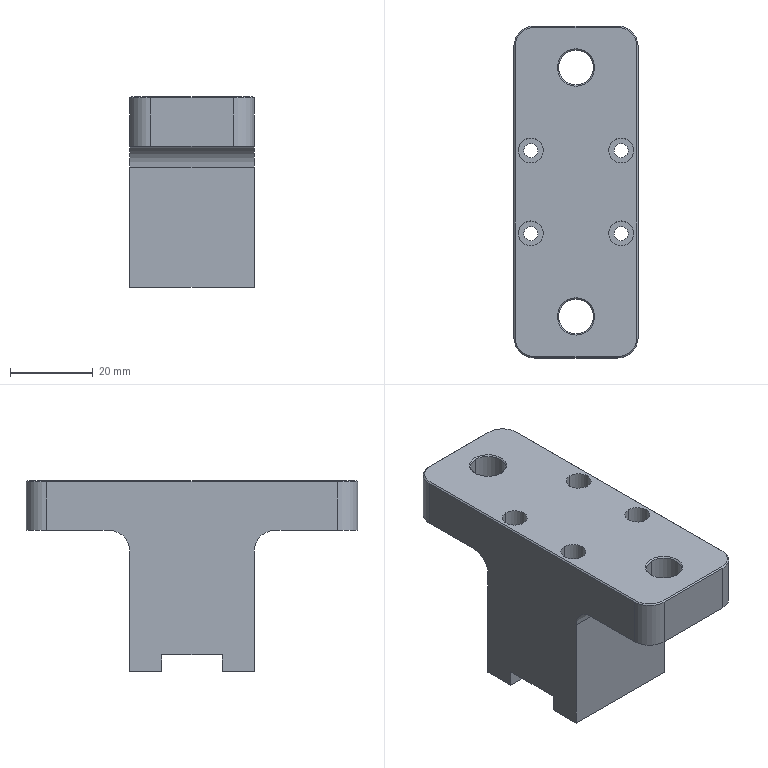NC program | NX | posted with a generic post | part box 30 x 80 x 46 mm
Lines 2546 to 3641 of 3641:
(ZLEVEL_PROFILE_COPY_1_COPY_COPY_1 , TOOL : D10JING)
N5060 T14 M6
N5062 G54
N5064 G17 G0 G90 X-36.665 Y21.884 S9500 M3
N5066 G43 Z30. H14
N5068 Z-14.333
N5070 G94 G1 Z-15.333 F1000.
N5072 X-35.866 Y20.5
N5074 G3 X-35. Y20. R1.
N5076 G1 X35. F1200.
N5078 G2 X45. Y10. R10.
N5080 G1 Y-10.
N5082 G2 X35. Y-20. R10.
N5084 G1 X-35.
N5086 G2 X-45. Y-10. R10.
N5088 G1 Y10.
N5090 G2 X-35. Y20. R10.
N5092 G3 X-34.134 Y20.5 R1.
N5094 G1 X-33.268 Y22.
N5096 Z-14.333
N5098 G0 X-36.665 Y21.884 Z-29.667
N5100 G1 Z-30.667 F1000.
N5102 X-35.866 Y20.5
N5104 G3 X-35. Y20. R1.
N5106 G1 X35. F1200.
N5108 G2 X45. Y10. R10.
N5110 G1 Y-10.
N5112 G2 X35. Y-20. R10.
N5114 G1 X-35.
N5116 G2 X-45. Y-10. R10.
N5118 G1 Y10.
N5120 G2 X-35. Y20. R10.
N5122 G3 X-34.134 Y20.5 R1.
N5124 G1 X-33.268 Y22.
N5126 Z-29.667
N5128 G0 X-36.665 Y21.884 Z-45.
N5130 G1 Z-46. F1000.
N5132 X-35.866 Y20.5
N5134 G3 X-35. Y20. R1.
N5136 G1 X35. F1200.
N5138 G2 X45. Y10. R10.
N5140 G1 Y-10.
N5142 G2 X35. Y-20. R10.
N5144 G1 X-35.
N5146 G2 X-45. Y-10. R10.
N5148 G1 Y10.
N5150 G2 X-35. Y20. R10.
N5152 G3 X-34.134 Y20.5 R1.
N5154 G1 X-33.268 Y22.
N5156 Z-45.
N5158 G0 Z30.
(ZLEVEL_PROFILE_COPY_1_COPY_COPY_1_COPY , TOOL : D10JING)
N5160 X-21.862 Y-21.911
N5162 Z-13.45
N5164 G1 Z-14.45 F1000.
N5166 X-20.499 Y-21.124
N5168 G3 X-19.999 Y-20.258 R1.
N5170 G1 X-20. Y-14.941 F1200.
N5172 Y10.081
N5174 X-19.999 Y20.258
N5176 G3 X-20.499 Y21.124 R1.
N5178 G1 X-21.86 Y21.91
N5180 Z-13.45
N5182 G0 X-21.864 Y-21.91 Z-27.9
N5184 G1 Z-28.9 F1000.
N5186 X-20.501 Y-21.124
N5188 G3 X-20.001 Y-20.258 R1.
N5190 G1 X-20. Y-14.941 F1200.
N5192 Y10.033
N5194 X-20.004 Y19.876
N5196 X-20.001 Y20.258
N5198 G3 X-20.493 Y21.128 R1.
N5200 G1 X-21.857 Y21.931
N5202 Z-27.9
N5204 G0 Z30.
N5206 X21.859 Y21.911
N5208 Z-13.45
N5210 G1 Z-14.45 F1000.
N5212 X20.497 Y21.124
N5214 G3 X19.997 Y20.258 R1.
N5216 G1 X20. Y15.002 F1200.
N5218 Y14.524
N5220 Y-15.
N5222 X19.997 Y-20.258
N5224 G3 X20.497 Y-21.124 R1.
N5226 G1 X21.859 Y-21.911
N5228 Z-13.45
N5230 G0 X21.86 Y21.91 Z-27.9
N5232 G1 Z-28.9 F1000.
N5234 X20.499 Y21.124
N5236 G3 X19.999 Y20.258 R1.
N5238 G1 X20. Y14.524 F1200.
N5240 Y-15.
N5242 X20.004 Y-15.767
N5244 X19.999 Y-20.258
N5246 G3 X20.498 Y-21.124 R1.
N5248 G1 X21.86 Y-21.913
N5250 Z-27.9
N5252 G0 Z30.
(FLOOR_WALL , TOOL : D10JING)
N5254 X39.997 Y22.001
N5256 Z-31.
N5258 G1 Z-34. F1250.
N5260 Y18.662
N5262 Y-18.662
N5264 G2 X35.165 Y-19.999 R10.
N5266 G1 Y19.999
N5268 X35. Y20.
N5270 X30.332
N5272 Y-20.
N5274 X25.5
N5276 Y20.
N5278 Y23.
N5280 Z-31.
N5282 G0 Z30.
N5284 X25.
N5286 Z-31.
N5288 G1 Z-34.
N5290 Y20.
N5292 Y-20.
N5294 Y-23.
N5296 Z-31.
N5298 G0 Z30.
N5300 X1.747 Y23.
N5302 Z-1.
N5304 G1 Z-4.
N5306 Y20.
N5308 Y-20.
N5310 X-1.75
N5312 Y20.
N5314 Y23.
N5316 Z-1.
N5318 G0 Z30.
N5320 X-2.25
N5322 Z-1.
N5324 G1 Z-4.
N5326 Y20.
N5328 Y-20.
N5330 Y-23.
N5332 X2.25
N5334 Y-20.
N5336 Y20.
N5338 Y23.
N5340 Z-1.
N5342 G0 Z30.
N5344 X-39.997 Y-22.001
N5346 Z-31.
N5348 G1 Z-34.
N5350 Y-18.662
N5352 Y18.662
N5354 G2 X-35.165 Y19.999 R10.
N5356 G1 Y-19.999
N5358 X-35. Y-20.
N5360 X-30.332
N5362 Y20.
N5364 X-25.5
N5366 Y-20.
N5368 Y-23.
N5370 Z-31.
N5372 G0 Z30.
N5374 X-25.
N5376 Z-31.
N5378 G1 Z-34.
N5380 Y-20.
N5382 Y20.
N5384 Y23.
N5386 Z-31.
N5388 G0 Z30.
N5390 M5
(ZLEVEL_PROFILE_1 , TOOL : D6R0.5)
N5392 T16 M6
N5394 G54
N5396 G17 G0 G90 X20.382 Y18.155 S9500 M3
N5398 G43 Z30. H16
N5400 Z-26.1
N5402 G94 G1 Z-29.1 F3500.
N5404 G3 X18. Y15.22 R3.
N5406 G1 Y-15.22
N5408 Y-15.238 Z-29.2
N5410 Y15.238
N5412 Y15.256 Z-29.3
N5414 Y-15.256
N5416 Y-15.274 Z-29.4
N5418 Y15.274
N5420 X18.001 Y15.292 Z-29.5
N5422 X18. Y14.856
N5424 Y-14.856
N5426 X18.001 Y-15.293
N5428 X18.01 Y-15.311 Z-29.6
N5430 X18.001 Y-15.
N5432 Y15.
N5434 X18.01 Y15.31
N5436 X18.018 Y15.328 Z-29.7
N5438 G2 X18.004 Y15. R1.796
N5440 G1 Y-15.
N5442 G2 X18.019 Y-15.329 R2.059
N5444 G1 X18.03 Y-15.348 Z-29.8
N5446 G3 X18.01 Y-15. R1.979
N5448 G1 Y15.
N5450 G3 X18.027 Y15.346 R1.617
N5452 G1 X18.038 Y15.365 Z-29.899
N5454 G2 X18.018 Y15. R1.824
N5456 G1 Y-15.
N5458 G2 X18.041 Y-15.367 R2.182
N5460 G1 X18.053 Y-15.386 Z-29.999
N5462 G3 X18.028 Y-15. R2.782
N5464 G1 Y15.
N5466 G3 X18.049 Y15.384 R2.335
N5468 G1 X18.066 Y15.401 Z-30.098
N5470 G2 X18.04 Y14.856 R3.839
N5472 G1 Y-14.856
N5474 G2 X18.071 Y-15.403 R5.117
N5476 G1 X18.091 Y-15.421 Z-30.197
N5478 G3 X18.054 Y-14.817 R5.077
N5480 G1 Y14.774
N5482 G3 X18.087 Y15.419 R4.846
N5484 G1 X18.108 Y15.437 Z-30.296
N5486 G2 X18.071 Y14.773 R4.156
N5488 G1 Y-14.795
N5490 G2 X18.113 Y-15.439 R4.852
N5492 G1 X18.135 Y-15.456 Z-30.394
N5494 G3 X18.09 Y-14.794 R4.325
N5496 G1 Y14.772
N5498 G3 X18.131 Y15.455 R4.004
N5500 G1 X18.154 Y15.473 Z-30.492
N5502 G2 X18.111 Y14.793 R3.764
N5504 G1 Y-14.815
N5506 G2 X18.157 Y-15.474 R3.78
N5508 G1 X18.179 Y-15.492 Z-30.589
N5510 G3 X18.134 Y-14.814 R3.969
N5512 G1 Y14.813
N5514 G3 X18.177 Y15.49 R3.697
N5516 G1 X18.204 Y15.5 Z-30.685
N5518 G2 X18.159 Y14.77 R4.729
N5520 G1 Y-14.791
N5522 G2 X18.206 Y-15.5 R4.542
N5524 G1 X18.222 Z-30.733
N5526 X18.238 Z-30.781
N5528 G3 X18.186 Y-14.769 R4.31
N5530 G1 Y14.769
N5532 G3 X18.236 Y15.5 R4.051
N5534 G1 X18.25 Z-30.829
N5536 X18.269 Z-30.877
N5538 G2 X18.216 Y14.734 R4.239
N5540 G1 Y-14.743
N5542 G2 X18.27 Y-15.5 R4.23
N5544 G1 X18.281 Z-30.924
N5546 X18.302 Z-30.972
N5548 G3 X18.247 Y-14.745 R3.522
N5550 G1 Y14.736
N5552 G3 X18.301 Y15.5 R3.844
N5554 G1 X18.311 Z-31.019
N5556 X18.333 Z-31.066
N5558 G2 X18.281 Y14.739 R3.671
N5560 G1 Y-14.747
N5562 X18.304 Y-14.856
N5564 G2 X18.333 Y-15.5 R6.898
N5566 G1 X18.345 Z-31.112
N5568 X18.364 Z-31.159
N5570 G3 X18.327 Y-14.766 R5.34
N5572 G1 X18.317 Y-14.749
N5574 Y14.742
N5576 X18.326 Y14.76
N5578 G3 X18.364 Y15.5 R5.553
N5580 G1 X18.386 Z-31.205
N5582 X18.406 Z-31.251
N5584 G2 X18.355 Y14.746 R4.818
N5586 G1 Y-14.734
N5588 G2 X18.406 Y-15.5 R5.15
N5590 G1 X18.428 Z-31.297
N5592 X18.447 Z-31.343
N5594 G3 X18.395 Y-14.737 R4.674
N5596 G1 Y14.733
N5598 G3 X18.447 Y15.5 R4.771
N5600 G1 X18.469 Z-31.388
N5602 X18.488 Z-31.433
N5604 G2 X18.436 Y14.736 R4.76
N5606 G1 Y-14.739
N5608 G2 X18.488 Y-15.5 R4.696
N5610 G1 X18.509 Z-31.478
N5612 X18.528 Z-31.523
N5614 G3 X18.488 Y-14.775 R5.453
N5616 G1 X18.48 Y-14.758
N5618 Y14.757
N5620 G3 X18.528 Y15.5 R3.899
N5622 G1 X18.549 Z-31.567
N5624 X18.577 Z-31.611
N5626 G2 X18.526 Y14.761 R5.321
N5628 G1 Y-14.761
N5630 G2 X18.577 Y-15.5 R5.311
N5632 G1 X18.602 Z-31.655
N5634 X18.629 Z-31.699
N5636 G3 X18.574 Y-14.759 R4.303
N5638 G1 Y14.759
N5640 G3 X18.629 Y15.5 R4.304
N5642 G1 X18.654 Z-31.742
N5644 X18.68 Z-31.785
N5646 G2 X18.623 Y14.739 R4.32
N5648 G1 Y-14.739
N5650 G2 X18.68 Y-15.5 R4.319
N5652 G1 X18.706 Z-31.828
N5654 X18.732 Z-31.87
N5656 G3 X18.675 Y-14.733 R4.453
N5658 G1 Y14.733
N5660 G3 X18.732 Y15.5 R4.453
N5662 G1 X18.757 Z-31.912
N5664 X18.787 Z-31.954
N5666 G2 X18.728 Y14.741 R3.922
N5668 G1 Y-14.741
N5670 G2 X18.787 Y-15.5 R3.922
N5672 G1 X18.808 Z-31.996
N5674 X18.84 Z-32.037
N5676 G3 X18.784 Y-14.735 R3.973
N5678 G1 Y14.735
N5680 G3 X18.84 Y15.5 R3.973
N5682 G1 X18.865 Z-32.078
N5684 X18.896 Z-32.119
N5686 X18.864 Y14.856
N5688 X18.84 Y14.728
N5690 Y-14.728
N5692 X18.864 Y-14.856
N5694 X18.896 Y-15.5
N5696 X18.929 Z-32.159
N5698 X18.962 Z-32.199
N5700 G3 X18.899 Y-14.724 R4.085
N5702 G1 Y14.724
N5704 G3 X18.962 Y15.5 R4.085
N5706 G1 X18.991 Z-32.238
N5708 X19.026 Z-32.278
N5710 G2 X18.96 Y14.72 R3.821
N5712 G1 Y-14.72
N5714 G2 X19.026 Y-15.5 R3.821
N5716 G1 X19.052 Z-32.317
N5718 X19.09 Z-32.355
N5720 G3 X19.022 Y-14.73 R3.637
N5722 G1 Y14.73
N5724 G3 X19.09 Y15.5 R3.636
N5726 G1 X19.112 Z-32.393
N5728 X19.152 Z-32.431
N5730 G2 X19.086 Y14.726 R3.585
N5732 G1 Y-14.726
N5734 G2 X19.152 Y-15.5 R3.585
N5736 G1 X19.174 Z-32.469
N5738 X19.213 Z-32.506
N5740 G3 X19.151 Y-14.722 R3.762
N5742 G1 Y14.722
N5744 G3 X19.213 Y15.5 R3.762
N5746 G1 X19.248 Z-32.542
N5748 X19.284 Z-32.579
N5750 X19.247 Y14.856
N5752 X19.218 Y14.705
N5754 Y-14.705
N5756 X19.247 Y-14.856
N5758 X19.284 Y-15.5
N5760 X19.32 Z-32.615
N5762 X19.357 Z-32.65
N5764 X19.321 Y-14.856
N5766 X19.287 Y-14.704
N5768 Y14.704
N5770 X19.321 Y14.856
N5772 X19.357 Y15.5
N5774 X19.391 Z-32.685
N5776 X19.428 Z-32.72
N5778 X19.394 Y14.856
N5780 X19.357 Y14.702
N5782 Y-14.702
N5784 X19.394 Y-14.856
N5786 X19.428 Y-15.5
N5788 X19.46 Z-32.754
N5790 X19.497 Z-32.789
N5792 X19.465 Y-14.856
N5794 X19.428 Y-14.7
N5796 Y14.7
N5798 X19.465 Y14.856
N5800 X19.497 Y15.5
N5802 X19.527 Z-32.822
N5804 X19.565 Z-32.855
N5806 G2 X19.501 Y14.698 R3.826
N5808 G1 Y-14.698
N5810 G2 X19.565 Y-15.5 R3.826
N5812 G1 X19.607 Z-32.888
N5814 X19.647 Z-32.92
N5816 G3 X19.576 Y-14.695 R3.918
N5818 G1 Y14.695
N5820 G3 X19.647 Y15.5 R3.918
N5822 G1 X19.689 Z-32.952
N5824 X19.727 Z-32.983
N5826 G2 X19.651 Y14.672 R3.791
N5828 G1 Y-14.672
N5830 G2 X19.727 Y-15.5 R3.791
N5832 G1 X19.768 Z-33.014
N5834 X19.806 Z-33.045
N5836 G3 X19.728 Y-14.663 R3.795
N5838 G1 Y14.663
N5840 G3 X19.806 Y15.5 R3.795
N5842 G1 X19.846 Z-33.075
N5844 X19.882 Z-33.105
N5846 G2 X19.806 Y14.668 R3.908
N5848 G1 Y-14.668
N5850 G2 X19.882 Y-15.5 R3.908
N5852 G1 X19.921 Z-33.134
N5854 X19.965 Z-33.163
N5856 X19.897 Y-14.727
N5858 X19.885 Y-14.699
N5860 Y14.699
N5862 X19.897 Y14.727
N5864 X19.965 Y15.5
N5866 X20.001 Z-33.191
N5868 X20.054 Z-33.219
N5870 G2 X19.966 Y14.68 R3.24
N5872 G1 Y-14.68
N5874 G2 X20.054 Y-15.5 R3.24
N5876 G1 X20.092 Z-33.246
N5878 X20.14 Z-33.273
N5880 G3 X20.047 Y-14.642 R3.349
N5882 G1 Y14.642
N5884 G3 X20.14 Y15.5 R3.349
N5886 G1 X20.18 Z-33.299
N5888 X20.223 Z-33.325
N5890 G2 X20.129 Y14.62 R3.483
N5892 G1 Y-14.62
N5894 G2 X20.223 Y-15.5 R3.483
N5896 G1 X20.265 Z-33.35
N5898 X20.311 Z-33.375
N5900 G3 X20.212 Y-14.616 R3.773
N5902 G1 Y14.616
N5904 G3 X20.311 Y15.5 R3.756
N5906 G1 X20.346 Z-33.399
N5908 X20.403 Z-33.423
N5910 X20.333 Y14.76
N5912 X20.296 Y14.648
N5914 Y-14.648
N5916 X20.334 Y-14.76
N5918 X20.403 Y-15.5
N5920 X20.405 Z-33.435
N5922 X20.425 Z-33.446
N5924 X20.449 Z-33.458
N5926 X20.492 Z-33.47
N5928 G3 X20.38 Y-14.631 R2.593
N5930 G1 Y14.631
N5932 G3 X20.492 Y15.5 R2.591
N5934 G1 X20.524 Z-33.492
N5936 X20.576 Z-33.514
N5938 G2 X20.466 Y14.597 R2.868
N5940 G1 Y-14.597
N5942 G2 X20.576 Y-15.5 R2.871
N5944 G1 X20.62 Z-33.535
N5946 X20.667 Z-33.556
N5948 X20.575 Y-14.609
N5950 X20.551 Y-14.562
N5952 Y14.562
N5954 X20.575 Y14.609
N5956 X20.667 Y15.5
N5958 X20.712 Z-33.576
N5960 X20.759 Z-33.596
N5962 X20.68 Y14.664
N5964 X20.637 Y14.551
N5966 Y-14.551
N5968 X20.68 Y-14.665
N5970 X20.759 Y-15.5
N5972 X20.799 Z-33.615
N5974 X20.847 Z-33.635
N5976 X20.771 Y-14.653
N5978 X20.724 Y-14.565
N5980 Y14.568
N5982 X20.771 Y14.653
N5984 X20.847 Y15.5
N5986 X20.882 Z-33.653
N5988 X20.93 Z-33.671
N5990 G2 X20.811 Y14.571 R2.721
N5992 G1 Y-14.566
N5994 G2 X20.93 Y-15.5 R2.744
N5996 G1 X20.977 Z-33.688
N5998 X21.028 Z-33.705
N6000 X20.937 Y-14.629
N6002 X20.897 Y-14.554
N6004 Y14.548
N6006 X20.938 Y14.634
N6008 X21.03 Y15.5
N6010 X21.083 Z-33.721
N6012 X21.132 Z-33.737
N6014 G2 X20.984 Y14.5 R3.187
N6016 G1 Y-14.5
N6018 G2 X21.128 Y-15.5 R3.108
N6020 G1 X21.178 Z-33.752
N6022 X21.222 Z-33.767
N6024 G3 X21.07 Y-14.465 R3.164
N6026 G1 Y14.465
N6028 G3 X21.227 Y15.5 R3.271
N6030 G1 X21.273 Z-33.78
N6032 X21.319 Z-33.794
N6034 G2 X21.155 Y14.463 R3.396
N6036 G1 Y-14.463
N6038 G2 X21.311 Y-15.5 R3.194
N6040 G1 X21.351 Z-33.807
N6042 X21.412 Z-33.82
N6044 G3 X21.239 Y-14.471 R2.87
N6046 G1 Y14.471
N6048 G3 X21.423 Y15.5 R3.036
N6050 G1 X21.436 Z-33.831
N6052 X21.519 Z-33.843
N6054 G2 X21.321 Y14.475 R2.403
N6056 G1 Y-14.475
N6058 G2 X21.504 Y-15.5 R2.294
N6060 G1 X21.527 Z-33.853
N6062 X21.588 Z-33.864
N6064 G3 X21.402 Y-14.447 R2.286
N6066 G1 Y14.444
N6068 G3 X21.606 Y15.5 R2.421
N6070 G1 X21.647 Z-33.873
N6072 X21.693 Z-33.883
N6074 X21.548 Y14.51
N6076 X21.48 Y14.389
N6078 Y-14.393
N6080 X21.546 Y-14.51
N6082 X21.667 Y-15.5
N6084 X21.71 Z-33.892
N6086 X21.752 Z-33.9
N6088 X21.627 Y-14.51
N6090 X21.557 Y-14.366
N6092 Y14.36
N6094 X21.63 Y14.51
N6096 X21.781 Y15.5
N6098 X21.82 Z-33.908
N6100 X21.859 Z-33.915
N6102 X21.717 Y14.51
N6104 X21.632 Y14.358
N6106 Y-14.367
N6108 X21.712 Y-14.51
N6110 X21.827 Y-15.5
N6112 X21.857 Z-33.922
N6114 X21.894 Z-33.929
N6116 X21.793 Y-14.51
N6118 X21.705 Y-14.375
N6120 Y14.364
N6122 G3 X21.929 Y15.5 R2.537
N6124 G1 X22.058 Y15.413 Z-33.95
N6126 G2 X21.831 Y14.417 R2.517
N6128 G1 Y-14.44
N6130 G2 X21.999 Y-15.487 R2.285
N6132 G3 X23.383 Y-17.095 R1.5
N6134 G1 X24.747 Y-17.197
N6136 Z-30.95
N6138 G0 Z30.
N6140 X-20.382 Y-18.155
N6142 Z-26.1
N6144 G1 Z-29.1
N6146 G3 X-18. Y-15.22 R3.
N6148 G1 Y15.22
N6150 Y15.238 Z-29.2
N6152 Y-15.238
N6154 Y-15.256 Z-29.3
N6156 Y15.256
N6158 Y15.274 Z-29.4
N6160 Y-15.274
N6162 X-18.001 Y-15.292 Z-29.5
N6164 X-18. Y-14.856
N6166 Y14.856
N6168 X-18.001 Y15.293
N6170 X-18.01 Y15.311 Z-29.6
N6172 X-18.001 Y15.
N6174 Y-15.
N6176 X-18.01 Y-15.31
N6178 X-18.018 Y-15.328 Z-29.7
N6180 G2 X-18.004 Y-15. R1.798
N6182 G1 Y15.
N6184 G2 X-18.019 Y15.329 R2.059
N6186 G1 X-18.03 Y15.348 Z-29.8
N6188 G3 X-18.01 Y15. R1.979
N6190 G1 Y-15.
N6192 G3 X-18.027 Y-15.346 R1.617
N6194 G1 X-18.038 Y-15.365 Z-29.899
N6196 G2 X-18.018 Y-15. R1.824
N6198 G1 Y15.
N6200 G2 X-18.041 Y15.367 R2.182
N6202 G1 X-18.053 Y15.386 Z-29.999
N6204 G3 X-18.028 Y15. R2.782
N6206 G1 Y-15.
N6208 G3 X-18.049 Y-15.384 R2.335
N6210 G1 X-18.066 Y-15.401 Z-30.098
N6212 G2 X-18.04 Y-14.856 R3.839
N6214 G1 Y14.856
N6216 G2 X-18.071 Y15.403 R5.117
N6218 G1 X-18.091 Y15.421 Z-30.197
N6220 G3 X-18.054 Y14.795 R5.976
N6222 G1 Y-14.774
N6224 G3 X-18.087 Y-15.419 R4.846
N6226 G1 X-18.108 Y-15.437 Z-30.296
N6228 G2 X-18.071 Y-14.773 R4.156
N6230 G1 Y14.795
N6232 G2 X-18.113 Y15.439 R4.852
N6234 G1 X-18.135 Y15.456 Z-30.394
N6236 G3 X-18.09 Y14.794 R4.325
N6238 G1 Y-14.772
N6240 G3 X-18.131 Y-15.455 R4.004
N6242 G1 X-18.154 Y-15.473 Z-30.492
N6244 G2 X-18.111 Y-14.793 R3.764
N6246 G1 Y14.815
N6248 G2 X-18.157 Y15.474 R3.78
N6250 G1 X-18.179 Y15.492 Z-30.589
N6252 G3 X-18.134 Y14.814 R3.969
N6254 G1 Y-14.813
N6256 G3 X-18.177 Y-15.49 R3.697
N6258 G1 X-18.204 Y-15.5 Z-30.685
N6260 G2 X-18.159 Y-14.77 R4.729
N6262 G1 Y14.791
N6264 G2 X-18.206 Y15.5 R4.542
N6266 G1 X-18.222 Z-30.733
N6268 X-18.238 Z-30.781
N6270 G3 X-18.186 Y14.769 R4.31
N6272 G1 Y-14.769
N6274 G3 X-18.236 Y-15.5 R4.051
N6276 G1 X-18.25 Z-30.829
N6278 X-18.269 Z-30.877
N6280 G2 X-18.216 Y-14.734 R4.239
N6282 G1 Y14.743
N6284 G2 X-18.27 Y15.5 R4.23
N6286 G1 X-18.281 Z-30.924
N6288 X-18.302 Z-30.972
N6290 G3 X-18.247 Y14.745 R3.522
N6292 G1 Y-14.736
N6294 G3 X-18.301 Y-15.5 R3.844
N6296 G1 X-18.311 Z-31.019
N6298 X-18.333 Z-31.066
N6300 G2 X-18.281 Y-14.739 R3.671
N6302 G1 Y14.747
N6304 X-18.304 Y14.856
N6306 G2 X-18.333 Y15.5 R6.898
N6308 G1 X-18.345 Z-31.112
N6310 X-18.364 Z-31.159
N6312 G3 X-18.327 Y14.766 R5.34
N6314 G1 X-18.317 Y14.749
N6316 Y-14.742
N6318 X-18.326 Y-14.76
N6320 G3 X-18.364 Y-15.5 R5.553
N6322 G1 X-18.386 Z-31.205
N6324 X-18.406 Z-31.251
N6326 G2 X-18.355 Y-14.746 R4.813
N6328 G1 Y14.734
N6330 G2 X-18.406 Y15.5 R5.15
N6332 G1 X-18.428 Z-31.297
N6334 X-18.447 Z-31.343
N6336 G3 X-18.395 Y14.737 R4.674
N6338 G1 Y-14.733
N6340 G3 X-18.447 Y-15.5 R4.771
N6342 G1 X-18.469 Z-31.388
N6344 X-18.488 Z-31.433
N6346 G2 X-18.436 Y-14.736 R4.76
N6348 G1 Y14.739
N6350 G2 X-18.488 Y15.5 R4.696
N6352 G1 X-18.509 Z-31.478
N6354 X-18.528 Z-31.523
N6356 G3 X-18.488 Y14.775 R5.453
N6358 G1 X-18.48 Y14.758
N6360 Y-14.757
N6362 G3 X-18.528 Y-15.5 R3.899
N6364 G1 X-18.549 Z-31.567
N6366 X-18.577 Z-31.611
N6368 G2 X-18.526 Y-14.761 R5.321
N6370 G1 Y14.761
N6372 G2 X-18.577 Y15.5 R5.311
N6374 G1 X-18.602 Z-31.655
N6376 X-18.629 Z-31.699
N6378 G3 X-18.574 Y14.759 R4.303
N6380 G1 Y-14.759
N6382 G3 X-18.629 Y-15.5 R4.304
N6384 G1 X-18.654 Z-31.742
N6386 X-18.68 Z-31.785
N6388 G2 X-18.623 Y-14.739 R4.32
N6390 G1 Y14.739
N6392 G2 X-18.68 Y15.5 R4.319
N6394 G1 X-18.706 Z-31.828
N6396 X-18.732 Z-31.87
N6398 G3 X-18.675 Y14.733 R4.453
N6400 G1 Y-14.733
N6402 G3 X-18.732 Y-15.5 R4.453
N6404 G1 X-18.757 Z-31.912
N6406 X-18.787 Z-31.954
N6408 G2 X-18.728 Y-14.741 R3.922
N6410 G1 Y14.741
N6412 G2 X-18.787 Y15.5 R3.922
N6414 G1 X-18.808 Z-31.996
N6416 X-18.84 Z-32.037
N6418 G3 X-18.784 Y14.735 R3.973
N6420 G1 Y-14.735
N6422 G3 X-18.84 Y-15.5 R3.973
N6424 G1 X-18.865 Z-32.078
N6426 X-18.896 Z-32.119
N6428 X-18.864 Y-14.856
N6430 X-18.84 Y-14.728
N6432 Y14.728
N6434 X-18.864 Y14.856
N6436 X-18.896 Y15.5
N6438 X-18.929 Z-32.159
N6440 X-18.962 Z-32.199
N6442 G3 X-18.899 Y14.724 R4.085
N6444 G1 Y-14.724
N6446 G3 X-18.962 Y-15.5 R4.085
N6448 G1 X-18.991 Z-32.238
N6450 X-19.026 Z-32.278
N6452 G2 X-18.96 Y-14.72 R3.821
N6454 G1 Y14.72
N6456 G2 X-19.026 Y15.5 R3.821
N6458 G1 X-19.052 Z-32.317
N6460 X-19.09 Z-32.355
N6462 G3 X-19.022 Y14.73 R3.642
N6464 G1 Y-14.73
N6466 G3 X-19.09 Y-15.5 R3.642
N6468 G1 X-19.112 Z-32.393
N6470 X-19.152 Z-32.431
N6472 G2 X-19.086 Y-14.726 R3.585
N6474 G1 Y14.726
N6476 G2 X-19.152 Y15.5 R3.585
N6478 G1 X-19.174 Z-32.469
N6480 X-19.213 Z-32.506
N6482 G3 X-19.151 Y14.722 R3.762
N6484 G1 Y-14.722
N6486 G3 X-19.213 Y-15.5 R3.762
N6488 G1 X-19.248 Z-32.542
N6490 X-19.284 Z-32.579
N6492 X-19.247 Y-14.856
N6494 X-19.218 Y-14.705
N6496 Y14.705
N6498 X-19.247 Y14.856
N6500 X-19.284 Y15.5
N6502 X-19.32 Z-32.615
N6504 X-19.357 Z-32.65
N6506 X-19.321 Y14.856
N6508 X-19.287 Y14.704
N6510 Y-14.704
N6512 X-19.321 Y-14.856
N6514 X-19.357 Y-15.5
N6516 X-19.391 Z-32.685
N6518 X-19.428 Z-32.72
N6520 X-19.394 Y-14.856
N6522 X-19.357 Y-14.702
N6524 Y14.702
N6526 X-19.394 Y14.856
N6528 X-19.428 Y15.5
N6530 X-19.46 Z-32.754
N6532 X-19.497 Z-32.789
N6534 X-19.465 Y14.856
N6536 X-19.428 Y14.7
N6538 Y-14.7
N6540 X-19.465 Y-14.856
N6542 X-19.497 Y-15.5
N6544 X-19.527 Z-32.822
N6546 X-19.565 Z-32.855
N6548 G2 X-19.501 Y-14.698 R3.826
N6550 G1 Y14.698
N6552 G2 X-19.565 Y15.5 R3.826
N6554 G1 X-19.607 Z-32.888
N6556 X-19.647 Z-32.92
N6558 G3 X-19.576 Y14.695 R3.918
N6560 G1 Y-14.695
N6562 G3 X-19.647 Y-15.5 R3.918
N6564 G1 X-19.689 Z-32.952
N6566 X-19.727 Z-32.983
N6568 G2 X-19.651 Y-14.672 R3.791
N6570 G1 Y14.672
N6572 G2 X-19.727 Y15.5 R3.791
N6574 G1 X-19.768 Z-33.014
N6576 X-19.806 Z-33.045
N6578 G3 X-19.728 Y14.663 R3.795
N6580 G1 Y-14.663
N6582 G3 X-19.806 Y-15.5 R3.795
N6584 G1 X-19.846 Z-33.075
N6586 X-19.882 Z-33.105
N6588 G2 X-19.806 Y-14.668 R3.908
N6590 G1 Y14.668
N6592 G2 X-19.882 Y15.5 R3.908
N6594 G1 X-19.921 Z-33.134
N6596 X-19.965 Z-33.163
N6598 X-19.897 Y14.727
N6600 X-19.885 Y14.699
N6602 Y-14.699
N6604 X-19.897 Y-14.727
N6606 X-19.965 Y-15.5
N6608 X-20.001 Z-33.191
N6610 X-20.054 Z-33.219
N6612 G2 X-19.966 Y-14.68 R3.24
N6614 G1 Y14.68
N6616 G2 X-20.054 Y15.5 R3.24
N6618 G1 X-20.092 Z-33.246
N6620 X-20.14 Z-33.273
N6622 G3 X-20.047 Y14.642 R3.349
N6624 G1 Y-14.642
N6626 G3 X-20.14 Y-15.5 R3.349
N6628 G1 X-20.18 Z-33.299
N6630 X-20.223 Z-33.325
N6632 G2 X-20.129 Y-14.62 R3.483
N6634 G1 Y14.62
N6636 G2 X-20.223 Y15.5 R3.483
N6638 G1 X-20.265 Z-33.35
N6640 X-20.311 Z-33.375
N6642 G3 X-20.212 Y14.616 R3.773
N6644 G1 Y-14.616
N6646 G3 X-20.311 Y-15.5 R3.756
N6648 G1 X-20.346 Z-33.399
N6650 X-20.403 Z-33.423
N6652 X-20.333 Y-14.76
N6654 X-20.296 Y-14.647
N6656 Y14.647
N6658 X-20.334 Y14.76
N6660 X-20.403 Y15.5
N6662 X-20.405 Z-33.435
N6664 X-20.425 Z-33.446
N6666 X-20.449 Z-33.458
N6668 X-20.492 Z-33.47
N6670 G3 X-20.38 Y14.631 R2.593
N6672 G1 Y-14.631
N6674 G3 X-20.492 Y-15.5 R2.591
N6676 G1 X-20.524 Z-33.492
N6678 X-20.576 Z-33.514
N6680 G2 X-20.466 Y-14.597 R2.868
N6682 G1 Y14.597
N6684 G2 X-20.576 Y15.5 R2.871
N6686 G1 X-20.62 Z-33.535
N6688 X-20.667 Z-33.556
N6690 X-20.575 Y14.609
N6692 X-20.551 Y14.562
N6694 Y-14.562
N6696 X-20.575 Y-14.609
N6698 X-20.667 Y-15.5
N6700 X-20.712 Z-33.576
N6702 X-20.759 Z-33.596
N6704 X-20.674 Y-14.641
N6706 X-20.637 Y-14.551
N6708 Y14.551
N6710 X-20.68 Y14.665
N6712 X-20.759 Y15.5
N6714 X-20.799 Z-33.615
N6716 X-20.847 Z-33.635
N6718 X-20.771 Y14.653
N6720 X-20.724 Y14.565
N6722 Y-14.555
N6724 X-20.766 Y-14.63
N6726 X-20.847 Y-15.5
N6728 X-20.882 Z-33.653
N6730 X-20.93 Z-33.671
N6732 X-20.867 Y-14.698
N6734 X-20.811 Y-14.565
N6736 Y14.566
N6738 G2 X-20.93 Y15.5 R2.744
N6740 G1 X-20.977 Z-33.688
N6742 X-21.028 Z-33.705
N6744 X-20.937 Y14.629
N6746 X-20.897 Y14.554
N6748 Y-14.555
N6750 X-20.955 Y-14.736
N6752 X-21.03 Y-15.5
N6754 X-21.083 Z-33.721
N6756 X-21.132 Z-33.737
N6758 G2 X-20.984 Y-14.499 R3.189
N6760 G1 Y14.5
N6762 G2 X-21.128 Y15.5 R3.108
N6764 G1 X-21.178 Z-33.752
N6766 X-21.222 Z-33.767
N6768 G3 X-21.07 Y14.465 R3.164
N6770 G1 Y-14.465
N6772 G3 X-21.227 Y-15.5 R3.27
N6774 G1 X-21.273 Z-33.78
N6776 X-21.319 Z-33.794
N6778 G2 X-21.155 Y-14.463 R3.396
N6780 G1 Y14.463
N6782 G2 X-21.311 Y15.5 R3.193
N6784 G1 X-21.351 Z-33.807
N6786 X-21.412 Z-33.82
N6788 G3 X-21.239 Y14.471 R2.87
N6790 G1 Y-14.471
N6792 G3 X-21.423 Y-15.5 R3.036
N6794 G1 X-21.436 Z-33.831
N6796 X-21.519 Z-33.843
N6798 G2 X-21.321 Y-14.48 R2.36
N6800 G1 Y14.475
N6802 G2 X-21.504 Y15.5 R2.294
N6804 G1 X-21.527 Z-33.853
N6806 X-21.588 Z-33.864
N6808 G3 X-21.402 Y14.447 R2.286
N6810 G1 Y-14.434
N6812 G3 X-21.606 Y-15.5 R2.506
N6814 G1 X-21.647 Z-33.873
N6816 X-21.693 Z-33.883
N6818 X-21.548 Y-14.51
N6820 X-21.48 Y-14.39
N6822 Y14.393
N6824 X-21.546 Y14.51
N6826 X-21.667 Y15.5
N6828 X-21.71 Z-33.892
N6830 X-21.752 Z-33.9
N6832 X-21.627 Y14.51
N6834 X-21.557 Y14.366
N6836 Y-14.361
N6838 X-21.63 Y-14.51
N6840 X-21.781 Y-15.5
N6842 X-21.82 Z-33.908
N6844 X-21.859 Z-33.915
N6846 X-21.717 Y-14.51
N6848 X-21.683 Y-14.418
N6850 X-21.632 Y-14.348
N6852 Y14.367
N6854 X-21.712 Y14.51
N6856 X-21.827 Y15.5
N6858 X-21.857 Z-33.922
N6860 X-21.894 Z-33.929
N6862 G3 X-21.705 Y14.375 R2.442
N6864 G1 Y-14.364
N6866 G3 X-21.929 Y-15.5 R2.537
N6868 G1 X-22.058 Y-15.413 Z-33.95
N6870 G2 X-21.831 Y-14.417 R2.517
N6872 G1 Y14.44
N6874 G2 X-21.999 Y15.487 R2.285
N6876 G3 X-23.383 Y17.095 R1.5
N6878 G1 X-24.747 Y17.197
N6880 Z-30.95
N6882 G0 Z30.
N6884 M5
(DRILLING_COPY_1 , TOOL : D6A45)
N6886 T01 M6
N6888 G54
N6890 G17 G0 G90 X-30. Y0. S5000 M3
N6892 G43 Z30. H1
N6894 G94 G81 G98 Z-35.8 F350. R-31.
N6896 X-10. Y-10.9 Z-1.8 R3.
N6898 Y10.9
N6900 X10.
N6902 Y-10.9
N6904 X30. Y0. Z-35.8 R-31.
N6906 G80
N6908 G0 X30. Y0. Z30.
N6910 M5
(DRILLING_COPY_1_COPY , TOOL : 3.4ZT)
N6912 T03 M6
N6914 G54
N6916 G17 G0 G90 X-10. Y10.9 S2000 M3
N6918 G43 Z30. H3
N6920 G94 G83 G98 Z-49.021 F100. Q2. R3.
N6922 X10.
N6924 Y-10.9
N6926 X-10.
N6928 G80
N6930 G0 X-10. Y-10.9 Z30.
N6932 M5
(DRILLING_COPY_1_COPY_COPY , TOOL : 8.4ZT)
N6934 T20 M6
N6936 G54
N6938 G17 G0 G90 X-30. Y0. S2000 M3
N6940 G43 Z30. H20
N6942 G94 G83 G98 Z-50.024 F100. Q2. R-31.
N6944 X30.
N6946 G80
N6948 G0 X30. Y0. Z30.
N6950 M5
(PLANAR_MILL_COPY_COPY_COPY_COPY_COPY_COPY_1_COPY_1 , TOOL : D6A45)
N6952 T01 M6
N6954 G54
N6956 G17 G0 G90 X9.134 Y-11.4 S9500 M3
N6958 G43 Z30. H1
N6960 Z0.5
N6962 G94 G1 Z-1. F1250.
N6964 G3 X10. Y-11.9 R1.
N6966 X11. Y-10.9 R1.
N6968 X10. Y-11.9 R-1.
N6970 X10.866 Y-11.4 R1.
N6972 G1 Z0.5
N6974 G0 Z30.
N6976 X16.2 Y0.866
N6978 Z0.5
N6980 G1 Z-1.
N6982 G3 X15.7 Y0. R1.
N6984 G1 Y-15.
N6986 G2 X15. Y-15.7 R0.7
N6988 G1 X7.25
N6990 G2 X6.55 Y-15. R0.7
N6992 G1 Y15.
N6994 G2 X7.25 Y15.7 R0.7
N6996 G1 X15.
N6998 G2 X15.7 Y15. R0.7
N7000 G1 Y0.
N7002 G3 X16.2 Y-0.866 R1.
N7004 G1 Z0.5
N7006 G0 Z30.
N7008 X10.866 Y11.4
N7010 Z0.5
N7012 G1 Z-1.
N7014 G3 X10. Y11.9 R1.
N7016 X9. Y10.9 R1.
N7018 X10. Y11.9 R-1.
N7020 X9.134 Y11.4 R1.
N7022 G1 Z0.5
N7024 G0 Z30.
N7026 X-9.134
N7028 Z0.5
N7030 G1 Z-1.
N7032 G3 X-10. Y11.9 R1.
N7034 X-11. Y10.9 R1.
N7036 X-10. Y11.9 R-1.
N7038 X-10.866 Y11.4 R1.
N7040 G1 Z0.5
N7042 G0 Z30.
N7044 X-16.2 Y-0.866
N7046 Z0.5
N7048 G1 Z-1.
N7050 G3 X-15.7 Y0. R1.
N7052 G1 Y15.
N7054 G2 X-15. Y15.7 R0.7
N7056 G1 X-7.25
N7058 G2 X-6.55 Y15. R0.7
N7060 G1 Y-15.
N7062 G2 X-7.25 Y-15.7 R0.7
N7064 G1 X-15.
N7066 G2 X-15.7 Y-15. R0.7
N7068 G1 Y0.
N7070 G3 X-16.2 Y0.866 R1.
N7072 G1 Z0.5
N7074 G0 Z30.
N7076 X-10.866 Y-11.4
N7078 Z0.5
N7080 G1 Z-1.
N7082 G3 X-10. Y-11.9 R1.
N7084 X-9. Y-10.9 R1.
N7086 X-10. Y-11.9 R-1.
N7088 X-9.134 Y-11.4 R1.
N7090 G1 Z0.5
N7092 G0 Z30.
(PLANAR_MILL_COPY_COPY_COPY_COPY_COPY_COPY_1_COPY_1_COPY , TOOL : D6A45)
N7094 X31.538 Y-1.71
N7096 Z-33.5
N7098 G1 Z-35.
N7100 X33. Y-0.866
N7102 G3 X33.5 Y0. R1.
N7104 X30. Y3.5 R3.5
N7106 X33.5 Y0. R-3.5
N7108 X33. Y0.866 R1.
N7110 G1 X31.538 Y1.71
N7112 Z-33.5
N7114 G0 Z30.
N7116 X24.22 Y17.069
N7118 Z-33.5
N7120 G1 Z-35.
N7122 X23.746 Y16.649
N7124 G3 X23.429 Y15.7 R1.
N7126 G1 X35.
N7128 G2 X40.7 Y10. R5.7
N7130 G1 Y-10.
N7132 G2 X35. Y-15.7 R5.7
N7134 G1 X23.429
N7136 G3 X23.746 Y-16.649 R1.
N7138 G1 X24.22 Y-17.069
N7140 Z-33.5
N7142 G0 Z30.
N7144 X-24.22
N7146 Z-33.5
N7148 G1 Z-35.
N7150 X-23.746 Y-16.649
N7152 G3 X-23.429 Y-15.7 R1.
N7154 G1 X-35.
N7156 G2 X-40.7 Y-10. R5.7
N7158 G1 Y10.
N7160 G2 X-35. Y15.7 R5.7
N7162 G1 X-23.429
N7164 G3 X-23.746 Y16.649 R1.
N7166 G1 X-24.22 Y17.069
N7168 Z-33.5
N7170 G0 Z30.
N7172 X-31.538 Y1.71
N7174 Z-33.5
N7176 G1 Z-35.
N7178 X-33. Y0.866
N7180 G3 X-33.5 Y0. R1.
N7182 X-30. Y-3.5 R3.5
N7184 X-33.5 Y0. R-3.5
N7186 X-33. Y-0.866 R1.
N7188 G1 X-31.538 Y-1.71
N7190 Z-33.5
N7192 G0 Z30.
N7194 M5
N7196 M2